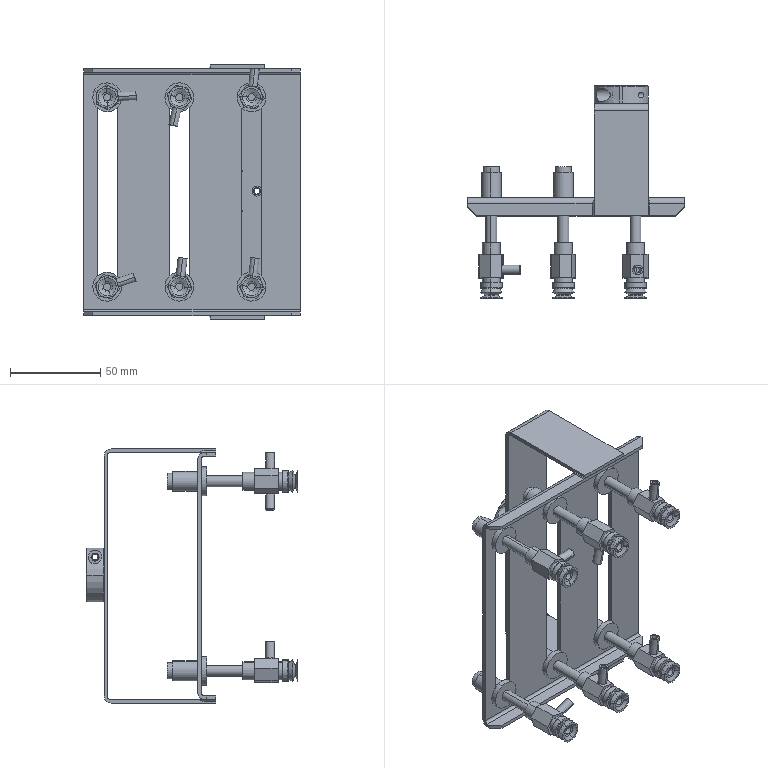Part | STEP file | Mobile suction-cup manipulator | 19 solids | 487 faces | box 120 x 117.5 x 141 mm | volume 84416 mm3 | plane 165 | cylinder 148 | cone 102 | spline 72 | commonest cylinder face diameters 10 x24 11 x18 3 x16 12 x15 5 x12 6 x12